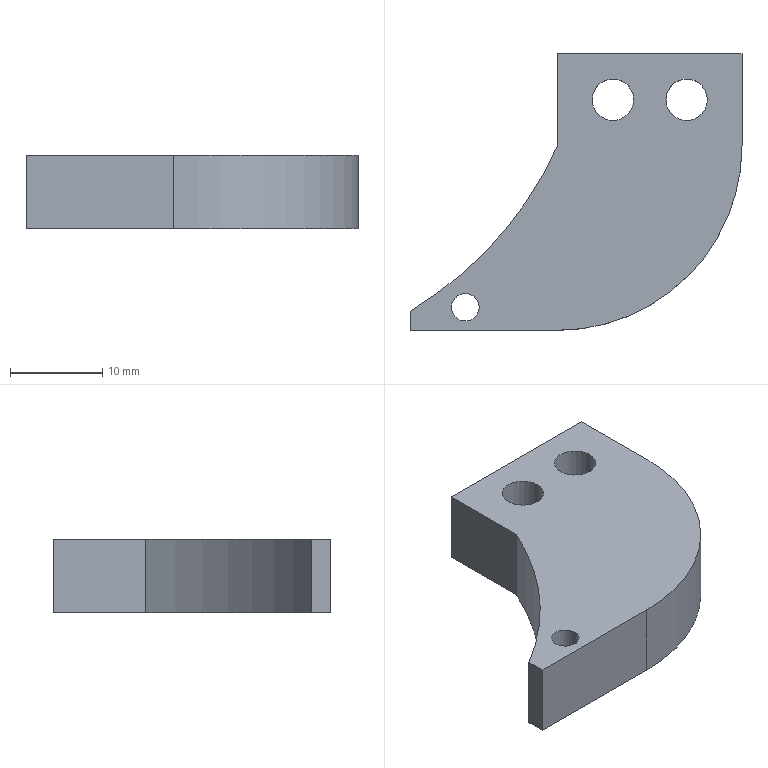Part | SolidWorks | features Extrusion 1, ICE 1 | 1 solid | 15 faces | box 36 x 30 x 8 mm | volume 4978 mm3 | cylinder 8 | plane 7 | commonest cylinder face diameters 4.5 x4 3 x2 40 x1 79.874 x1
STEP:
#1=CARTESIAN_POINT('',(-15.18,-18.932,8.));
#2=VERTEX_POINT('',#1);
#3=CARTESIAN_POINT('',(-18.18,-18.932,8.));
#4=VERTEX_POINT('',#3);
#5=CARTESIAN_POINT('',(-16.68,-18.932,8.));
#6=DIRECTION('',(0.,0.,-1.));
#7=DIRECTION('',(-1.,0.,0.));
#8=AXIS2_PLACEMENT_3D('',#5,#6,#7);
#9=CIRCLE('',#8,1.5);
#10=EDGE_CURVE('',#2,#4,#9,.T.);
#11=ORIENTED_EDGE('',*,*,#10,.F.);
#12=CARTESIAN_POINT('',(-15.18,-18.932,0.));
#13=VERTEX_POINT('',#12);
#14=CARTESIAN_POINT('',(-15.18,-18.932,8.));
#15=DIRECTION('',(0.,0.,-1.));
#16=VECTOR('',#15,1000.);
#17=LINE('',#14,#16);
#18=EDGE_CURVE('',#2,#13,#17,.T.);
#19=ORIENTED_EDGE('',*,*,#18,.T.);
#20=CARTESIAN_POINT('',(-18.18,-18.932,0.));
#21=VERTEX_POINT('',#20);
#22=CARTESIAN_POINT('',(-16.68,-18.932,0.));
#23=DIRECTION('',(0.,0.,-1.));
#24=DIRECTION('',(-1.,0.,0.));
#25=AXIS2_PLACEMENT_3D('',#22,#23,#24);
#26=CIRCLE('',#25,1.5);
#27=EDGE_CURVE('',#13,#21,#26,.T.);
#28=ORIENTED_EDGE('',*,*,#27,.T.);
#29=CARTESIAN_POINT('',(-18.18,-18.932,8.));
#30=DIRECTION('',(0.,0.,-1.));
#31=VECTOR('',#30,1000.);
#32=LINE('',#29,#31);
#33=EDGE_CURVE('',#4,#21,#32,.T.);
#34=ORIENTED_EDGE('',*,*,#33,.F.);
#35=EDGE_LOOP('',(#11,#19,#28,#34));
#36=FACE_OUTER_BOUND('',#35,.T.);
#37=CARTESIAN_POINT('',(-16.68,-18.932,8.));
#38=DIRECTION('',(0.,0.,-1.));
#39=DIRECTION('',(-1.,0.,0.));
#40=AXIS2_PLACEMENT_3D('',#37,#38,#39);
#41=CYLINDRICAL_SURFACE('',#40,1.5);
#42=ADVANCED_FACE('',(#36),#41,.F.);
#43=CARTESIAN_POINT('',(1.57,3.568,8.));
#44=VERTEX_POINT('',#43);
#45=CARTESIAN_POINT('',(-2.93,3.568,8.));
#46=VERTEX_POINT('',#45);
#47=CARTESIAN_POINT('',(-0.6805,3.568,8.));
#48=DIRECTION('',(0.,0.,-1.));
#49=DIRECTION('',(-1.,0.,0.));
#50=AXIS2_PLACEMENT_3D('',#47,#48,#49);
#51=CIRCLE('',#50,2.25);
#52=EDGE_CURVE('',#44,#46,#51,.T.);
#53=ORIENTED_EDGE('',*,*,#52,.F.);
#54=CARTESIAN_POINT('',(1.57,3.568,0.));
#55=VERTEX_POINT('',#54);
#56=CARTESIAN_POINT('',(1.57,3.568,8.));
#57=DIRECTION('',(0.,0.,-1.));
#58=VECTOR('',#57,1000.);
#59=LINE('',#56,#58);
#60=EDGE_CURVE('',#44,#55,#59,.T.);
#61=ORIENTED_EDGE('',*,*,#60,.T.);
#62=CARTESIAN_POINT('',(-2.93,3.568,0.));
#63=VERTEX_POINT('',#62);
#64=CARTESIAN_POINT('',(-0.6805,3.568,0.));
#65=DIRECTION('',(0.,0.,-1.));
#66=DIRECTION('',(-1.,0.,0.));
#67=AXIS2_PLACEMENT_3D('',#64,#65,#66);
#68=CIRCLE('',#67,2.25);
#69=EDGE_CURVE('',#55,#63,#68,.T.);
#70=ORIENTED_EDGE('',*,*,#69,.T.);
#71=CARTESIAN_POINT('',(-2.93,3.568,8.));
#72=DIRECTION('',(0.,0.,-1.));
#73=VECTOR('',#72,1000.);
#74=LINE('',#71,#73);
#75=EDGE_CURVE('',#46,#63,#74,.T.);
#76=ORIENTED_EDGE('',*,*,#75,.F.);
#77=EDGE_LOOP('',(#53,#61,#70,#76));
#78=FACE_OUTER_BOUND('',#77,.T.);
#79=CARTESIAN_POINT('',(-0.6805,3.568,8.));
#80=DIRECTION('',(0.,0.,-1.));
#81=DIRECTION('',(-1.,0.,0.));
#82=AXIS2_PLACEMENT_3D('',#79,#80,#81);
#83=CYLINDRICAL_SURFACE('',#82,2.25);
#84=ADVANCED_FACE('',(#78),#83,.F.);
#85=CARTESIAN_POINT('',(9.57,3.568,8.));
#86=VERTEX_POINT('',#85);
#87=CARTESIAN_POINT('',(5.07,3.568,8.));
#88=VERTEX_POINT('',#87);
#89=CARTESIAN_POINT('',(7.32,3.568,8.));
#90=DIRECTION('',(0.,0.,-1.));
#91=DIRECTION('',(-1.,0.,0.));
#92=AXIS2_PLACEMENT_3D('',#89,#90,#91);
#93=CIRCLE('',#92,2.25);
#94=EDGE_CURVE('',#86,#88,#93,.T.);
#95=ORIENTED_EDGE('',*,*,#94,.F.);
#96=CARTESIAN_POINT('',(9.57,3.568,0.));
#97=VERTEX_POINT('',#96);
#98=CARTESIAN_POINT('',(9.57,3.568,8.));
#99=DIRECTION('',(0.,0.,-1.));
#100=VECTOR('',#99,1000.);
#101=LINE('',#98,#100);
#102=EDGE_CURVE('',#86,#97,#101,.T.);
#103=ORIENTED_EDGE('',*,*,#102,.T.);
#104=CARTESIAN_POINT('',(5.07,3.568,0.));
#105=VERTEX_POINT('',#104);
#106=CARTESIAN_POINT('',(7.32,3.568,0.));
#107=DIRECTION('',(0.,0.,-1.));
#108=DIRECTION('',(-1.,0.,0.));
#109=AXIS2_PLACEMENT_3D('',#106,#107,#108);
#110=CIRCLE('',#109,2.25);
#111=EDGE_CURVE('',#97,#105,#110,.T.);
#112=ORIENTED_EDGE('',*,*,#111,.T.);
#113=CARTESIAN_POINT('',(5.07,3.568,8.));
#114=DIRECTION('',(0.,0.,-1.));
#115=VECTOR('',#114,1000.);
#116=LINE('',#113,#115);
#117=EDGE_CURVE('',#88,#105,#116,.T.);
#118=ORIENTED_EDGE('',*,*,#117,.F.);
#119=EDGE_LOOP('',(#95,#103,#112,#118));
#120=FACE_OUTER_BOUND('',#119,.T.);
#121=CARTESIAN_POINT('',(7.32,3.568,8.));
#122=DIRECTION('',(0.,0.,-1.));
#123=DIRECTION('',(-1.,0.,0.));
#124=AXIS2_PLACEMENT_3D('',#121,#122,#123);
#125=CYLINDRICAL_SURFACE('',#124,2.25);
#126=ADVANCED_FACE('',(#120),#125,.F.);
#127=CARTESIAN_POINT('',(-6.68,8.568,0.));
#128=VERTEX_POINT('',#127);
#129=CARTESIAN_POINT('',(-6.68,-1.432,0.));
#130=VERTEX_POINT('',#129);
#131=CARTESIAN_POINT('',(-6.68,8.568,0.));
#132=DIRECTION('',(0.,-1.,0.));
#133=VECTOR('',#132,1000.);
#134=LINE('',#131,#133);
#135=EDGE_CURVE('',#128,#130,#134,.T.);
#136=ORIENTED_EDGE('',*,*,#135,.T.);
#137=CARTESIAN_POINT('',(-6.68,-1.432,8.));
#138=VERTEX_POINT('',#137);
#139=CARTESIAN_POINT('',(-6.68,-1.432,8.));
#140=DIRECTION('',(0.,0.,-1.));
#141=VECTOR('',#140,1000.);
#142=LINE('',#139,#141);
#143=EDGE_CURVE('',#138,#130,#142,.T.);
#144=ORIENTED_EDGE('',*,*,#143,.F.);
#145=CARTESIAN_POINT('',(-6.68,8.568,8.));
#146=VERTEX_POINT('',#145);
#147=CARTESIAN_POINT('',(-6.68,8.568,8.));
#148=DIRECTION('',(0.,-1.,0.));
#149=VECTOR('',#148,1000.);
#150=LINE('',#147,#149);
#151=EDGE_CURVE('',#146,#138,#150,.T.);
#152=ORIENTED_EDGE('',*,*,#151,.F.);
#153=CARTESIAN_POINT('',(-6.68,8.568,8.));
#154=DIRECTION('',(0.,0.,-1.));
#155=VECTOR('',#154,1000.);
#156=LINE('',#153,#155);
#157=EDGE_CURVE('',#146,#128,#156,.T.);
#158=ORIENTED_EDGE('',*,*,#157,.T.);
#159=EDGE_LOOP('',(#136,#144,#152,#158));
#160=FACE_OUTER_BOUND('',#159,.T.);
#161=CARTESIAN_POINT('',(-6.68,8.568,8.));
#162=DIRECTION('',(1.,0.,0.));
#163=DIRECTION('',(0.,0.,-1.));
#164=AXIS2_PLACEMENT_3D('',#161,#162,#163);
#165=PLANE('',#164);
#166=ADVANCED_FACE('',(#160),#165,.F.);
#167=CARTESIAN_POINT('',(-22.68,-19.349,0.));
#168=VERTEX_POINT('',#167);
#169=CARTESIAN_POINT('',(-43.09,14.978,0.));
#170=DIRECTION('',(0.,0.,-1.));
#171=DIRECTION('',(1.,0.,0.));
#172=AXIS2_PLACEMENT_3D('',#169,#170,#171);
#173=CIRCLE('',#172,39.937);
#174=EDGE_CURVE('',#130,#168,#173,.T.);
#175=ORIENTED_EDGE('',*,*,#174,.T.);
#176=CARTESIAN_POINT('',(-22.68,-19.349,8.));
#177=VERTEX_POINT('',#176);
#178=CARTESIAN_POINT('',(-22.68,-19.349,8.));
#179=DIRECTION('',(0.,0.,-1.));
#180=VECTOR('',#179,1000.);
#181=LINE('',#178,#180);
#182=EDGE_CURVE('',#177,#168,#181,.T.);
#183=ORIENTED_EDGE('',*,*,#182,.F.);
#184=CARTESIAN_POINT('',(-43.09,14.978,8.));
#185=DIRECTION('',(0.,0.,-1.));
#186=DIRECTION('',(1.,0.,0.));
#187=AXIS2_PLACEMENT_3D('',#184,#185,#186);
#188=CIRCLE('',#187,39.937);
#189=EDGE_CURVE('',#138,#177,#188,.T.);
#190=ORIENTED_EDGE('',*,*,#189,.F.);
#191=ORIENTED_EDGE('',*,*,#143,.T.);
#192=EDGE_LOOP('',(#175,#183,#190,#191));
#193=FACE_OUTER_BOUND('',#192,.T.);
#194=CARTESIAN_POINT('',(-43.09,14.978,8.));
#195=DIRECTION('',(0.,0.,-1.));
#196=DIRECTION('',(-1.,0.,0.));
#197=AXIS2_PLACEMENT_3D('',#194,#195,#196);
#198=CYLINDRICAL_SURFACE('',#197,39.937);
#199=ADVANCED_FACE('',(#193),#198,.F.);
#200=CARTESIAN_POINT('',(-22.68,-21.432,0.));
#201=VERTEX_POINT('',#200);
#202=CARTESIAN_POINT('',(-22.68,-21.432,0.));
#203=DIRECTION('',(0.,-1.,0.));
#204=VECTOR('',#203,1000.);
#205=LINE('',#202,#204);
#206=EDGE_CURVE('',#168,#201,#205,.T.);
#207=ORIENTED_EDGE('',*,*,#206,.T.);
#208=CARTESIAN_POINT('',(-22.68,-21.432,8.));
#209=VERTEX_POINT('',#208);
#210=CARTESIAN_POINT('',(-22.68,-21.432,8.));
#211=DIRECTION('',(0.,0.,-1.));
#212=VECTOR('',#211,1000.);
#213=LINE('',#210,#212);
#214=EDGE_CURVE('',#209,#201,#213,.T.);
#215=ORIENTED_EDGE('',*,*,#214,.F.);
#216=CARTESIAN_POINT('',(-22.68,-21.432,8.));
#217=DIRECTION('',(0.,-1.,0.));
#218=VECTOR('',#217,1000.);
#219=LINE('',#216,#218);
#220=EDGE_CURVE('',#177,#209,#219,.T.);
#221=ORIENTED_EDGE('',*,*,#220,.F.);
#222=ORIENTED_EDGE('',*,*,#182,.T.);
#223=EDGE_LOOP('',(#207,#215,#221,#222));
#224=FACE_OUTER_BOUND('',#223,.T.);
#225=CARTESIAN_POINT('',(-22.68,-21.432,8.));
#226=DIRECTION('',(1.,0.,0.));
#227=DIRECTION('',(0.,0.,-1.));
#228=AXIS2_PLACEMENT_3D('',#225,#226,#227);
#229=PLANE('',#228);
#230=ADVANCED_FACE('',(#224),#229,.F.);
#231=CARTESIAN_POINT('',(-6.68,-21.432,0.));
#232=VERTEX_POINT('',#231);
#233=CARTESIAN_POINT('',(-6.68,-21.432,0.));
#234=DIRECTION('',(1.,0.,0.));
#235=VECTOR('',#234,1000.);
#236=LINE('',#233,#235);
#237=EDGE_CURVE('',#201,#232,#236,.T.);
#238=ORIENTED_EDGE('',*,*,#237,.T.);
#239=CARTESIAN_POINT('',(-6.68,-21.432,8.));
#240=VERTEX_POINT('',#239);
#241=CARTESIAN_POINT('',(-6.68,-21.432,8.));
#242=DIRECTION('',(0.,0.,-1.));
#243=VECTOR('',#242,1000.);
#244=LINE('',#241,#243);
#245=EDGE_CURVE('',#240,#232,#244,.T.);
#246=ORIENTED_EDGE('',*,*,#245,.F.);
#247=CARTESIAN_POINT('',(-6.68,-21.432,8.));
#248=DIRECTION('',(1.,0.,0.));
#249=VECTOR('',#248,1000.);
#250=LINE('',#247,#249);
#251=EDGE_CURVE('',#209,#240,#250,.T.);
#252=ORIENTED_EDGE('',*,*,#251,.F.);
#253=ORIENTED_EDGE('',*,*,#214,.T.);
#254=EDGE_LOOP('',(#238,#246,#252,#253));
#255=FACE_OUTER_BOUND('',#254,.T.);
#256=CARTESIAN_POINT('',(-6.68,-21.432,8.));
#257=DIRECTION('',(0.,1.,0.));
#258=DIRECTION('',(0.,0.,1.));
#259=AXIS2_PLACEMENT_3D('',#256,#257,#258);
#260=PLANE('',#259);
#261=ADVANCED_FACE('',(#255),#260,.F.);
#262=CARTESIAN_POINT('',(13.32,-1.432,0.));
#263=VERTEX_POINT('',#262);
#264=CARTESIAN_POINT('',(-6.68,-1.432,0.));
#265=DIRECTION('',(0.,0.,1.));
#266=DIRECTION('',(1.,0.,0.));
#267=AXIS2_PLACEMENT_3D('',#264,#265,#266);
#268=CIRCLE('',#267,20.);
#269=EDGE_CURVE('',#232,#263,#268,.T.);
#270=ORIENTED_EDGE('',*,*,#269,.T.);
#271=CARTESIAN_POINT('',(13.32,-1.432,8.));
#272=VERTEX_POINT('',#271);
#273=CARTESIAN_POINT('',(13.32,-1.432,8.));
#274=DIRECTION('',(0.,0.,-1.));
#275=VECTOR('',#274,1000.);
#276=LINE('',#273,#275);
#277=EDGE_CURVE('',#272,#263,#276,.T.);
#278=ORIENTED_EDGE('',*,*,#277,.F.);
#279=CARTESIAN_POINT('',(-6.68,-1.432,8.));
#280=DIRECTION('',(0.,0.,1.));
#281=DIRECTION('',(1.,0.,0.));
#282=AXIS2_PLACEMENT_3D('',#279,#280,#281);
#283=CIRCLE('',#282,20.);
#284=EDGE_CURVE('',#240,#272,#283,.T.);
#285=ORIENTED_EDGE('',*,*,#284,.F.);
#286=ORIENTED_EDGE('',*,*,#245,.T.);
#287=EDGE_LOOP('',(#270,#278,#285,#286));
#288=FACE_OUTER_BOUND('',#287,.T.);
#289=CARTESIAN_POINT('',(-6.68,-1.432,8.));
#290=DIRECTION('',(0.,0.,-1.));
#291=DIRECTION('',(-1.,0.,0.));
#292=AXIS2_PLACEMENT_3D('',#289,#290,#291);
#293=CYLINDRICAL_SURFACE('',#292,20.);
#294=ADVANCED_FACE('',(#288),#293,.T.);
#295=CARTESIAN_POINT('',(13.32,8.568,0.));
#296=VERTEX_POINT('',#295);
#297=CARTESIAN_POINT('',(13.32,8.568,0.));
#298=DIRECTION('',(0.,1.,0.));
#299=VECTOR('',#298,1000.);
#300=LINE('',#297,#299);
#301=EDGE_CURVE('',#263,#296,#300,.T.);
#302=ORIENTED_EDGE('',*,*,#301,.T.);
#303=CARTESIAN_POINT('',(13.32,8.568,8.));
#304=VERTEX_POINT('',#303);
#305=CARTESIAN_POINT('',(13.32,8.568,8.));
#306=DIRECTION('',(0.,0.,-1.));
#307=VECTOR('',#306,1000.);
#308=LINE('',#305,#307);
#309=EDGE_CURVE('',#304,#296,#308,.T.);
#310=ORIENTED_EDGE('',*,*,#309,.F.);
#311=CARTESIAN_POINT('',(13.32,8.568,8.));
#312=DIRECTION('',(0.,1.,0.));
#313=VECTOR('',#312,1000.);
#314=LINE('',#311,#313);
#315=EDGE_CURVE('',#272,#304,#314,.T.);
#316=ORIENTED_EDGE('',*,*,#315,.F.);
#317=ORIENTED_EDGE('',*,*,#277,.T.);
#318=EDGE_LOOP('',(#302,#310,#316,#317));
#319=FACE_OUTER_BOUND('',#318,.T.);
#320=CARTESIAN_POINT('',(13.32,8.568,8.));
#321=DIRECTION('',(-1.,0.,0.));
#322=DIRECTION('',(0.,-1.,0.));
#323=AXIS2_PLACEMENT_3D('',#320,#321,#322);
#324=PLANE('',#323);
#325=ADVANCED_FACE('',(#319),#324,.F.);
#326=CARTESIAN_POINT('',(-6.68,8.568,0.));
#327=DIRECTION('',(-1.,0.,0.));
#328=VECTOR('',#327,1000.);
#329=LINE('',#326,#328);
#330=EDGE_CURVE('',#296,#128,#329,.T.);
#331=ORIENTED_EDGE('',*,*,#330,.T.);
#332=ORIENTED_EDGE('',*,*,#157,.F.);
#333=CARTESIAN_POINT('',(-6.68,8.568,8.));
#334=DIRECTION('',(-1.,0.,0.));
#335=VECTOR('',#334,1000.);
#336=LINE('',#333,#335);
#337=EDGE_CURVE('',#304,#146,#336,.T.);
#338=ORIENTED_EDGE('',*,*,#337,.F.);
#339=ORIENTED_EDGE('',*,*,#309,.T.);
#340=EDGE_LOOP('',(#331,#332,#338,#339));
#341=FACE_OUTER_BOUND('',#340,.T.);
#342=CARTESIAN_POINT('',(-6.68,8.568,8.));
#343=DIRECTION('',(0.,-1.,0.));
#344=DIRECTION('',(0.,0.,-1.));
#345=AXIS2_PLACEMENT_3D('',#342,#343,#344);
#346=PLANE('',#345);
#347=ADVANCED_FACE('',(#341),#346,.F.);
#348=CARTESIAN_POINT('',(-16.68,-18.932,8.));
#349=DIRECTION('',(0.,0.,-1.));
#350=DIRECTION('',(-1.,0.,0.));
#351=AXIS2_PLACEMENT_3D('',#348,#349,#350);
#352=CIRCLE('',#351,1.5);
#353=EDGE_CURVE('',#4,#2,#352,.T.);
#354=ORIENTED_EDGE('',*,*,#353,.T.);
#355=ORIENTED_EDGE('',*,*,#10,.T.);
#356=EDGE_LOOP('',(#354,#355));
#357=FACE_BOUND('',#356,.T.);
#358=CARTESIAN_POINT('',(-0.6805,3.568,8.));
#359=DIRECTION('',(0.,0.,-1.));
#360=DIRECTION('',(-1.,0.,0.));
#361=AXIS2_PLACEMENT_3D('',#358,#359,#360);
#362=CIRCLE('',#361,2.25);
#363=EDGE_CURVE('',#46,#44,#362,.T.);
#364=ORIENTED_EDGE('',*,*,#363,.T.);
#365=ORIENTED_EDGE('',*,*,#52,.T.);
#366=EDGE_LOOP('',(#364,#365));
#367=FACE_BOUND('',#366,.T.);
#368=CARTESIAN_POINT('',(7.32,3.568,8.));
#369=DIRECTION('',(0.,0.,-1.));
#370=DIRECTION('',(-1.,0.,0.));
#371=AXIS2_PLACEMENT_3D('',#368,#369,#370);
#372=CIRCLE('',#371,2.25);
#373=EDGE_CURVE('',#88,#86,#372,.T.);
#374=ORIENTED_EDGE('',*,*,#373,.T.);
#375=ORIENTED_EDGE('',*,*,#94,.T.);
#376=EDGE_LOOP('',(#374,#375));
#377=FACE_BOUND('',#376,.T.);
#378=ORIENTED_EDGE('',*,*,#151,.T.);
#379=ORIENTED_EDGE('',*,*,#189,.T.);
#380=ORIENTED_EDGE('',*,*,#220,.T.);
#381=ORIENTED_EDGE('',*,*,#251,.T.);
#382=ORIENTED_EDGE('',*,*,#284,.T.);
#383=ORIENTED_EDGE('',*,*,#315,.T.);
#384=ORIENTED_EDGE('',*,*,#337,.T.);
#385=EDGE_LOOP('',(#378,#379,#380,#381,#382,#383,#384));
#386=FACE_OUTER_BOUND('',#385,.T.);
#387=CARTESIAN_POINT('',(-43.09,14.978,8.));
#388=DIRECTION('',(0.,0.,1.));
#389=DIRECTION('',(1.,0.,0.));
#390=AXIS2_PLACEMENT_3D('',#387,#388,#389);
#391=PLANE('',#390);
#392=ADVANCED_FACE('',(#357,#367,#377,#386),#391,.T.);
#393=CARTESIAN_POINT('',(-16.68,-18.932,0.));
#394=DIRECTION('',(0.,0.,-1.));
#395=DIRECTION('',(-1.,0.,0.));
#396=AXIS2_PLACEMENT_3D('',#393,#394,#395);
#397=CIRCLE('',#396,1.5);
#398=EDGE_CURVE('',#21,#13,#397,.T.);
#399=ORIENTED_EDGE('',*,*,#398,.F.);
#400=ORIENTED_EDGE('',*,*,#27,.F.);
#401=EDGE_LOOP('',(#399,#400));
#402=FACE_BOUND('',#401,.T.);
#403=CARTESIAN_POINT('',(-0.6805,3.568,0.));
#404=DIRECTION('',(0.,0.,-1.));
#405=DIRECTION('',(-1.,0.,0.));
#406=AXIS2_PLACEMENT_3D('',#403,#404,#405);
#407=CIRCLE('',#406,2.25);
#408=EDGE_CURVE('',#63,#55,#407,.T.);
#409=ORIENTED_EDGE('',*,*,#408,.F.);
#410=ORIENTED_EDGE('',*,*,#69,.F.);
#411=EDGE_LOOP('',(#409,#410));
#412=FACE_BOUND('',#411,.T.);
#413=CARTESIAN_POINT('',(7.32,3.568,0.));
#414=DIRECTION('',(0.,0.,-1.));
#415=DIRECTION('',(-1.,0.,0.));
#416=AXIS2_PLACEMENT_3D('',#413,#414,#415);
#417=CIRCLE('',#416,2.25);
#418=EDGE_CURVE('',#105,#97,#417,.T.);
#419=ORIENTED_EDGE('',*,*,#418,.F.);
#420=ORIENTED_EDGE('',*,*,#111,.F.);
#421=EDGE_LOOP('',(#419,#420));
#422=FACE_BOUND('',#421,.T.);
#423=ORIENTED_EDGE('',*,*,#135,.F.);
#424=ORIENTED_EDGE('',*,*,#330,.F.);
#425=ORIENTED_EDGE('',*,*,#301,.F.);
#426=ORIENTED_EDGE('',*,*,#269,.F.);
#427=ORIENTED_EDGE('',*,*,#237,.F.);
#428=ORIENTED_EDGE('',*,*,#206,.F.);
#429=ORIENTED_EDGE('',*,*,#174,.F.);
#430=EDGE_LOOP('',(#423,#424,#425,#426,#427,#428,#429));
#431=FACE_OUTER_BOUND('',#430,.T.);
#432=CARTESIAN_POINT('',(-43.09,14.978,0.));
#433=DIRECTION('',(0.,0.,1.));
#434=DIRECTION('',(1.,0.,0.));
#435=AXIS2_PLACEMENT_3D('',#432,#433,#434);
#436=PLANE('',#435);
#437=ADVANCED_FACE('',(#402,#412,#422,#431),#436,.F.);
#438=ORIENTED_EDGE('',*,*,#102,.F.);
#439=ORIENTED_EDGE('',*,*,#373,.F.);
#440=ORIENTED_EDGE('',*,*,#117,.T.);
#441=ORIENTED_EDGE('',*,*,#418,.T.);
#442=EDGE_LOOP('',(#438,#439,#440,#441));
#443=FACE_OUTER_BOUND('',#442,.T.);
#444=CARTESIAN_POINT('',(7.32,3.568,8.));
#445=DIRECTION('',(0.,0.,-1.));
#446=DIRECTION('',(-1.,0.,0.));
#447=AXIS2_PLACEMENT_3D('',#444,#445,#446);
#448=CYLINDRICAL_SURFACE('',#447,2.25);
#449=ADVANCED_FACE('',(#443),#448,.F.);
#450=ORIENTED_EDGE('',*,*,#60,.F.);
#451=ORIENTED_EDGE('',*,*,#363,.F.);
#452=ORIENTED_EDGE('',*,*,#75,.T.);
#453=ORIENTED_EDGE('',*,*,#408,.T.);
#454=EDGE_LOOP('',(#450,#451,#452,#453));
#455=FACE_OUTER_BOUND('',#454,.T.);
#456=CARTESIAN_POINT('',(-0.6805,3.568,8.));
#457=DIRECTION('',(0.,0.,-1.));
#458=DIRECTION('',(-1.,0.,0.));
#459=AXIS2_PLACEMENT_3D('',#456,#457,#458);
#460=CYLINDRICAL_SURFACE('',#459,2.25);
#461=ADVANCED_FACE('',(#455),#460,.F.);
#462=ORIENTED_EDGE('',*,*,#18,.F.);
#463=ORIENTED_EDGE('',*,*,#353,.F.);
#464=ORIENTED_EDGE('',*,*,#33,.T.);
#465=ORIENTED_EDGE('',*,*,#398,.T.);
#466=EDGE_LOOP('',(#462,#463,#464,#465));
#467=FACE_OUTER_BOUND('',#466,.T.);
#468=CARTESIAN_POINT('',(-16.68,-18.932,8.));
#469=DIRECTION('',(0.,0.,-1.));
#470=DIRECTION('',(-1.,0.,0.));
#471=AXIS2_PLACEMENT_3D('',#468,#469,#470);
#472=CYLINDRICAL_SURFACE('',#471,1.5);
#473=ADVANCED_FACE('',(#467),#472,.F.);
#474=CLOSED_SHELL('',(#42,#84,#126,#166,#199,#230,#261,#294,#325,#347,#392,#437,#449,#461,#473));
#475=MANIFOLD_SOLID_BREP('',#474);
#476=CARTESIAN_POINT('',(0.,0.,0.));
#477=DIRECTION('',(0.,0.,1.));
#478=DIRECTION('',(1.,0.,0.));
#479=AXIS2_PLACEMENT_3D('',#476,#477,#478);
#480=(LENGTH_UNIT()NAMED_UNIT(*)SI_UNIT(.MILLI.,.METRE.));
#481=UNCERTAINTY_MEASURE_WITH_UNIT(LENGTH_MEASURE(0.00001),#480,'','');
#482=(NAMED_UNIT(*)PLANE_ANGLE_UNIT()SI_UNIT($,.RADIAN.));
#483=(NAMED_UNIT(*)SI_UNIT($,.STERADIAN.)SOLID_ANGLE_UNIT());
#484=(GEOMETRIC_REPRESENTATION_CONTEXT(3)GLOBAL_UNCERTAINTY_ASSIGNED_CONTEXT((#481))GLOBAL_UNIT_ASSIGNED_CONTEXT((#480,#482,#483))REPRESENTATION_CONTEXT('',''));
#485=ADVANCED_BREP_SHAPE_REPRESENTATION('',(#475,#479),#484);